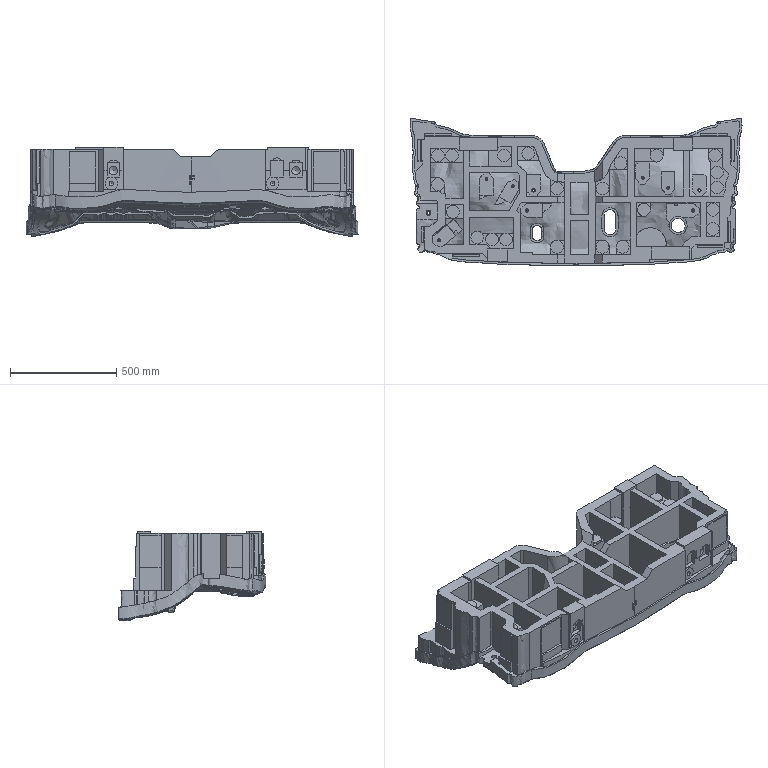Part | NX | features solid 2 | 1 solid | 4013 faces | volume 130884701 mm3 | spline 3396 | plane 500 | cylinder 103 | cone 12 | sphere 2 | commonest cylinder face diameters 60 x25 42 x13 20 x9 48 x6 7 x4 9 x4